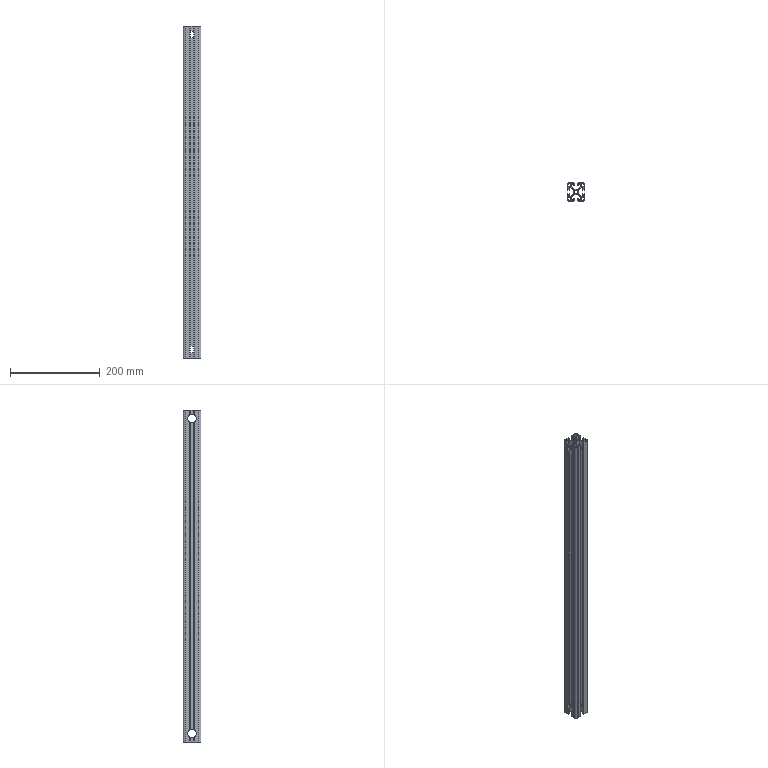Part | SolidWorks | features BaseBody 1, HoleWzd 1, MoveFace 1 | 1 solid | 235 faces | box 40 x 40 x 740 mm | volume 314551 mm3 | plane 166 | cylinder 69 | commonest cylinder face diameters 1.5 x18 2 x16 6.8 x15 19 x12 6.6 x4 9 x4